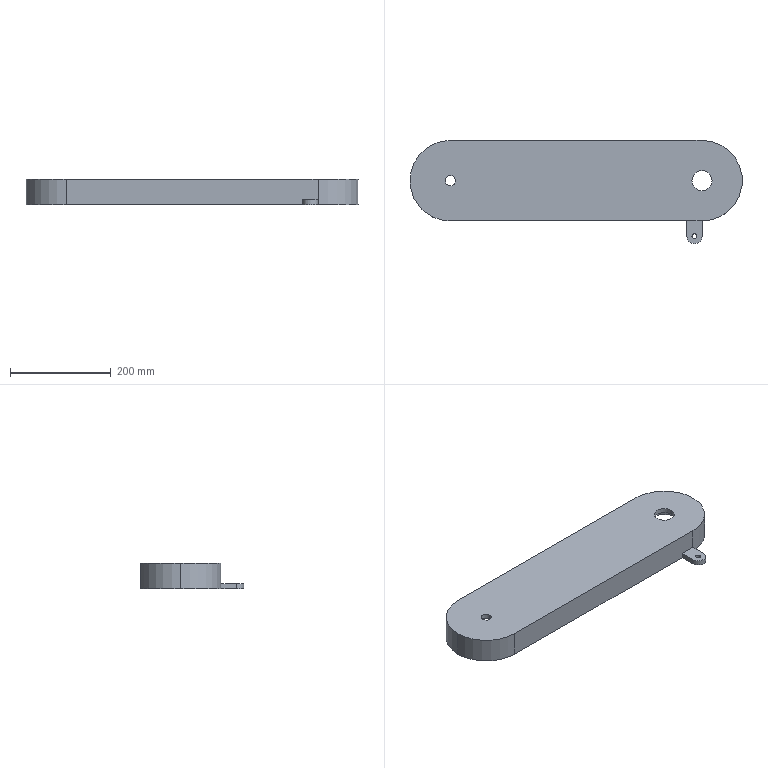Part | SolidWorks | features ICE 2, Extrusion 1 | 1 solid | 23 faces | box 660 x 205 x 50 mm | volume 1585598 mm3 | cylinder 13 | plane 10 | commonest cylinder face diameters 140 x3 160 x3 10 x2 20 x2 40 x2 30 x1
STEP:
#1=CARTESIAN_POINT('',(-10.,-110.,-30.));
#2=VERTEX_POINT('',#1);
#3=CARTESIAN_POINT('',(-20.,-110.,-30.));
#4=VERTEX_POINT('',#3);
#5=CARTESIAN_POINT('',(-15.,-110.,-30.));
#6=DIRECTION('',(0.,0.,-1.));
#7=DIRECTION('',(1.,0.,0.));
#8=AXIS2_PLACEMENT_3D('',#5,#6,#7);
#9=CIRCLE('',#8,5.);
#10=EDGE_CURVE('',#2,#4,#9,.T.);
#11=ORIENTED_EDGE('',*,*,#10,.F.);
#12=CARTESIAN_POINT('',(-10.,-110.,-40.));
#13=VERTEX_POINT('',#12);
#14=CARTESIAN_POINT('',(-10.,-110.,-30.));
#15=DIRECTION('',(0.,0.,-1.));
#16=VECTOR('',#15,1000.);
#17=LINE('',#14,#16);
#18=EDGE_CURVE('',#2,#13,#17,.T.);
#19=ORIENTED_EDGE('',*,*,#18,.T.);
#20=CARTESIAN_POINT('',(-20.,-110.,-40.));
#21=VERTEX_POINT('',#20);
#22=CARTESIAN_POINT('',(-15.,-110.,-40.));
#23=DIRECTION('',(0.,0.,-1.));
#24=DIRECTION('',(1.,0.,0.));
#25=AXIS2_PLACEMENT_3D('',#22,#23,#24);
#26=CIRCLE('',#25,5.);
#27=EDGE_CURVE('',#13,#21,#26,.T.);
#28=ORIENTED_EDGE('',*,*,#27,.T.);
#29=CARTESIAN_POINT('',(-20.,-110.,-30.));
#30=DIRECTION('',(0.,0.,-1.));
#31=VECTOR('',#30,1000.);
#32=LINE('',#29,#31);
#33=EDGE_CURVE('',#4,#21,#32,.T.);
#34=ORIENTED_EDGE('',*,*,#33,.F.);
#35=EDGE_LOOP('',(#11,#19,#28,#34));
#36=FACE_OUTER_BOUND('',#35,.T.);
#37=CARTESIAN_POINT('',(-15.,-110.,-30.));
#38=DIRECTION('',(0.,0.,-1.));
#39=DIRECTION('',(-1.,0.,0.));
#40=AXIS2_PLACEMENT_3D('',#37,#38,#39);
#41=CYLINDRICAL_SURFACE('',#40,5.);
#42=ADVANCED_FACE('',(#36),#41,.F.);
#43=CARTESIAN_POINT('',(0.,70.,-40.));
#44=VERTEX_POINT('',#43);
#45=CARTESIAN_POINT('',(70.,0.,-40.));
#46=VERTEX_POINT('',#45);
#47=CARTESIAN_POINT('',(0.,0.,-40.));
#48=DIRECTION('',(0.,0.,-1.));
#49=DIRECTION('',(-1.,0.,0.));
#50=AXIS2_PLACEMENT_3D('',#47,#48,#49);
#51=CIRCLE('',#50,70.);
#52=EDGE_CURVE('',#44,#46,#51,.T.);
#53=ORIENTED_EDGE('',*,*,#52,.T.);
#54=CARTESIAN_POINT('',(70.,0.,0.));
#55=VERTEX_POINT('',#54);
#56=CARTESIAN_POINT('',(70.,0.,-40.));
#57=DIRECTION('',(0.,0.,1.));
#58=VECTOR('',#57,1000.);
#59=LINE('',#56,#58);
#60=EDGE_CURVE('',#46,#55,#59,.T.);
#61=ORIENTED_EDGE('',*,*,#60,.T.);
#62=CARTESIAN_POINT('',(0.,70.,0.));
#63=VERTEX_POINT('',#62);
#64=CARTESIAN_POINT('',(0.,0.,0.));
#65=DIRECTION('',(0.,0.,-1.));
#66=DIRECTION('',(-1.,0.,0.));
#67=AXIS2_PLACEMENT_3D('',#64,#65,#66);
#68=CIRCLE('',#67,70.);
#69=EDGE_CURVE('',#63,#55,#68,.T.);
#70=ORIENTED_EDGE('',*,*,#69,.F.);
#71=CARTESIAN_POINT('',(0.,70.,-40.));
#72=DIRECTION('',(0.,0.,1.));
#73=VECTOR('',#72,1000.);
#74=LINE('',#71,#73);
#75=EDGE_CURVE('',#44,#63,#74,.T.);
#76=ORIENTED_EDGE('',*,*,#75,.F.);
#77=EDGE_LOOP('',(#53,#61,#70,#76));
#78=FACE_OUTER_BOUND('',#77,.T.);
#79=CARTESIAN_POINT('',(0.,0.,-40.));
#80=DIRECTION('',(0.,0.,1.));
#81=DIRECTION('',(1.,0.,0.));
#82=AXIS2_PLACEMENT_3D('',#79,#80,#81);
#83=CYLINDRICAL_SURFACE('',#82,70.);
#84=ADVANCED_FACE('',(#78),#83,.F.);
#85=CARTESIAN_POINT('',(-510.,0.,10.));
#86=VERTEX_POINT('',#85);
#87=CARTESIAN_POINT('',(-490.,0.,10.));
#88=VERTEX_POINT('',#87);
#89=CARTESIAN_POINT('',(-500.,0.,10.));
#90=DIRECTION('',(0.,0.,1.));
#91=DIRECTION('',(1.,0.,0.));
#92=AXIS2_PLACEMENT_3D('',#89,#90,#91);
#93=CIRCLE('',#92,10.);
#94=EDGE_CURVE('',#86,#88,#93,.T.);
#95=ORIENTED_EDGE('',*,*,#94,.T.);
#96=CARTESIAN_POINT('',(-490.,0.,0.));
#97=VERTEX_POINT('',#96);
#98=CARTESIAN_POINT('',(-490.,0.,10.));
#99=DIRECTION('',(0.,0.,-1.));
#100=VECTOR('',#99,1000.);
#101=LINE('',#98,#100);
#102=EDGE_CURVE('',#88,#97,#101,.T.);
#103=ORIENTED_EDGE('',*,*,#102,.T.);
#104=CARTESIAN_POINT('',(-510.,0.,0.));
#105=VERTEX_POINT('',#104);
#106=CARTESIAN_POINT('',(-500.,0.,0.));
#107=DIRECTION('',(0.,0.,1.));
#108=DIRECTION('',(1.,0.,0.));
#109=AXIS2_PLACEMENT_3D('',#106,#107,#108);
#110=CIRCLE('',#109,10.);
#111=EDGE_CURVE('',#105,#97,#110,.T.);
#112=ORIENTED_EDGE('',*,*,#111,.F.);
#113=CARTESIAN_POINT('',(-510.,0.,10.));
#114=DIRECTION('',(0.,0.,-1.));
#115=VECTOR('',#114,1000.);
#116=LINE('',#113,#115);
#117=EDGE_CURVE('',#86,#105,#116,.T.);
#118=ORIENTED_EDGE('',*,*,#117,.F.);
#119=EDGE_LOOP('',(#95,#103,#112,#118));
#120=FACE_OUTER_BOUND('',#119,.T.);
#121=CARTESIAN_POINT('',(-500.,0.,10.));
#122=DIRECTION('',(0.,0.,-1.));
#123=DIRECTION('',(-1.,0.,0.));
#124=AXIS2_PLACEMENT_3D('',#121,#122,#123);
#125=CYLINDRICAL_SURFACE('',#124,10.);
#126=ADVANCED_FACE('',(#120),#125,.F.);
#127=CARTESIAN_POINT('',(-20.,0.,10.));
#128=VERTEX_POINT('',#127);
#129=CARTESIAN_POINT('',(20.,0.,10.));
#130=VERTEX_POINT('',#129);
#131=CARTESIAN_POINT('',(0.,0.,10.));
#132=DIRECTION('',(0.,0.,1.));
#133=DIRECTION('',(1.,0.,0.));
#134=AXIS2_PLACEMENT_3D('',#131,#132,#133);
#135=CIRCLE('',#134,20.);
#136=EDGE_CURVE('',#128,#130,#135,.T.);
#137=ORIENTED_EDGE('',*,*,#136,.T.);
#138=CARTESIAN_POINT('',(20.,0.,0.));
#139=VERTEX_POINT('',#138);
#140=CARTESIAN_POINT('',(20.,0.,10.));
#141=DIRECTION('',(0.,0.,-1.));
#142=VECTOR('',#141,1000.);
#143=LINE('',#140,#142);
#144=EDGE_CURVE('',#130,#139,#143,.T.);
#145=ORIENTED_EDGE('',*,*,#144,.T.);
#146=CARTESIAN_POINT('',(-20.,0.,0.));
#147=VERTEX_POINT('',#146);
#148=CARTESIAN_POINT('',(0.,0.,0.));
#149=DIRECTION('',(0.,0.,1.));
#150=DIRECTION('',(1.,0.,0.));
#151=AXIS2_PLACEMENT_3D('',#148,#149,#150);
#152=CIRCLE('',#151,20.);
#153=EDGE_CURVE('',#147,#139,#152,.T.);
#154=ORIENTED_EDGE('',*,*,#153,.F.);
#155=CARTESIAN_POINT('',(-20.,0.,10.));
#156=DIRECTION('',(0.,0.,-1.));
#157=VECTOR('',#156,1000.);
#158=LINE('',#155,#157);
#159=EDGE_CURVE('',#128,#147,#158,.T.);
#160=ORIENTED_EDGE('',*,*,#159,.F.);
#161=EDGE_LOOP('',(#137,#145,#154,#160));
#162=FACE_OUTER_BOUND('',#161,.T.);
#163=CARTESIAN_POINT('',(0.,0.,10.));
#164=DIRECTION('',(0.,0.,-1.));
#165=DIRECTION('',(-1.,0.,0.));
#166=AXIS2_PLACEMENT_3D('',#163,#164,#165);
#167=CYLINDRICAL_SURFACE('',#166,20.);
#168=ADVANCED_FACE('',(#162),#167,.F.);
#169=CARTESIAN_POINT('',(-580.,0.,10.));
#170=VERTEX_POINT('',#169);
#171=CARTESIAN_POINT('',(-500.,-80.,10.));
#172=VERTEX_POINT('',#171);
#173=CARTESIAN_POINT('',(-500.,0.,10.));
#174=DIRECTION('',(0.,0.,1.));
#175=DIRECTION('',(1.,0.,0.));
#176=AXIS2_PLACEMENT_3D('',#173,#174,#175);
#177=CIRCLE('',#176,80.);
#178=EDGE_CURVE('',#170,#172,#177,.T.);
#179=ORIENTED_EDGE('',*,*,#178,.F.);
#180=CARTESIAN_POINT('',(-580.,0.,-40.));
#181=VERTEX_POINT('',#180);
#182=CARTESIAN_POINT('',(-580.,0.,10.));
#183=DIRECTION('',(0.,0.,-1.));
#184=VECTOR('',#183,1000.);
#185=LINE('',#182,#184);
#186=EDGE_CURVE('',#170,#181,#185,.T.);
#187=ORIENTED_EDGE('',*,*,#186,.T.);
#188=CARTESIAN_POINT('',(-500.,-80.,-40.));
#189=VERTEX_POINT('',#188);
#190=CARTESIAN_POINT('',(-500.,0.,-40.));
#191=DIRECTION('',(0.,0.,-1.));
#192=DIRECTION('',(-1.,0.,0.));
#193=AXIS2_PLACEMENT_3D('',#190,#191,#192);
#194=CIRCLE('',#193,80.);
#195=EDGE_CURVE('',#189,#181,#194,.T.);
#196=ORIENTED_EDGE('',*,*,#195,.F.);
#197=CARTESIAN_POINT('',(-500.,-80.,10.));
#198=DIRECTION('',(0.,0.,-1.));
#199=VECTOR('',#198,1000.);
#200=LINE('',#197,#199);
#201=EDGE_CURVE('',#172,#189,#200,.T.);
#202=ORIENTED_EDGE('',*,*,#201,.F.);
#203=EDGE_LOOP('',(#179,#187,#196,#202));
#204=FACE_OUTER_BOUND('',#203,.T.);
#205=CARTESIAN_POINT('',(-500.,0.,10.));
#206=DIRECTION('',(0.,0.,-1.));
#207=DIRECTION('',(-1.,0.,0.));
#208=AXIS2_PLACEMENT_3D('',#205,#206,#207);
#209=CYLINDRICAL_SURFACE('',#208,80.);
#210=ADVANCED_FACE('',(#204),#209,.T.);
#211=ORIENTED_EDGE('',*,*,#136,.F.);
#212=CARTESIAN_POINT('',(0.,0.,10.));
#213=DIRECTION('',(0.,0.,1.));
#214=DIRECTION('',(1.,0.,0.));
#215=AXIS2_PLACEMENT_3D('',#212,#213,#214);
#216=CIRCLE('',#215,20.);
#217=EDGE_CURVE('',#130,#128,#216,.T.);
#218=ORIENTED_EDGE('',*,*,#217,.F.);
#219=EDGE_LOOP('',(#211,#218));
#220=FACE_BOUND('',#219,.T.);
#221=CARTESIAN_POINT('',(0.,-80.,10.));
#222=VERTEX_POINT('',#221);
#223=CARTESIAN_POINT('',(0.,80.,10.));
#224=VERTEX_POINT('',#223);
#225=CARTESIAN_POINT('',(0.,0.,10.));
#226=DIRECTION('',(0.,0.,1.));
#227=DIRECTION('',(1.,0.,0.));
#228=AXIS2_PLACEMENT_3D('',#225,#226,#227);
#229=CIRCLE('',#228,80.);
#230=EDGE_CURVE('',#222,#224,#229,.T.);
#231=ORIENTED_EDGE('',*,*,#230,.T.);
#232=CARTESIAN_POINT('',(-500.,80.,10.));
#233=VERTEX_POINT('',#232);
#234=CARTESIAN_POINT('',(0.,80.,10.));
#235=DIRECTION('',(-1.,0.,0.));
#236=VECTOR('',#235,1000.);
#237=LINE('',#234,#236);
#238=EDGE_CURVE('',#224,#233,#237,.T.);
#239=ORIENTED_EDGE('',*,*,#238,.T.);
#240=CARTESIAN_POINT('',(-500.,0.,10.));
#241=DIRECTION('',(0.,0.,1.));
#242=DIRECTION('',(1.,0.,0.));
#243=AXIS2_PLACEMENT_3D('',#240,#241,#242);
#244=CIRCLE('',#243,80.);
#245=EDGE_CURVE('',#233,#170,#244,.T.);
#246=ORIENTED_EDGE('',*,*,#245,.T.);
#247=ORIENTED_EDGE('',*,*,#178,.T.);
#248=CARTESIAN_POINT('',(-500.,-80.,10.));
#249=DIRECTION('',(1.,0.,0.));
#250=VECTOR('',#249,1000.);
#251=LINE('',#248,#250);
#252=EDGE_CURVE('',#172,#222,#251,.T.);
#253=ORIENTED_EDGE('',*,*,#252,.T.);
#254=EDGE_LOOP('',(#231,#239,#246,#247,#253));
#255=FACE_OUTER_BOUND('',#254,.T.);
#256=ORIENTED_EDGE('',*,*,#94,.F.);
#257=CARTESIAN_POINT('',(-500.,0.,10.));
#258=DIRECTION('',(0.,0.,1.));
#259=DIRECTION('',(1.,0.,0.));
#260=AXIS2_PLACEMENT_3D('',#257,#258,#259);
#261=CIRCLE('',#260,10.);
#262=EDGE_CURVE('',#88,#86,#261,.T.);
#263=ORIENTED_EDGE('',*,*,#262,.F.);
#264=EDGE_LOOP('',(#256,#263));
#265=FACE_BOUND('',#264,.T.);
#266=CARTESIAN_POINT('',(0.,0.,10.));
#267=DIRECTION('',(0.,0.,1.));
#268=DIRECTION('',(1.,0.,0.));
#269=AXIS2_PLACEMENT_3D('',#266,#267,#268);
#270=PLANE('',#269);
#271=ADVANCED_FACE('',(#220,#255,#265),#270,.T.);
#272=CARTESIAN_POINT('',(-500.,70.,0.));
#273=VERTEX_POINT('',#272);
#274=CARTESIAN_POINT('',(-500.,70.,0.));
#275=DIRECTION('',(1.,0.,0.));
#276=VECTOR('',#275,1000.);
#277=LINE('',#274,#276);
#278=EDGE_CURVE('',#273,#63,#277,.T.);
#279=ORIENTED_EDGE('',*,*,#278,.T.);
#280=ORIENTED_EDGE('',*,*,#69,.T.);
#281=CARTESIAN_POINT('',(0.,-70.,0.));
#282=VERTEX_POINT('',#281);
#283=CARTESIAN_POINT('',(0.,0.,0.));
#284=DIRECTION('',(0.,0.,-1.));
#285=DIRECTION('',(-1.,0.,0.));
#286=AXIS2_PLACEMENT_3D('',#283,#284,#285);
#287=CIRCLE('',#286,70.);
#288=EDGE_CURVE('',#55,#282,#287,.T.);
#289=ORIENTED_EDGE('',*,*,#288,.T.);
#290=CARTESIAN_POINT('',(-500.,-70.,0.));
#291=VERTEX_POINT('',#290);
#292=CARTESIAN_POINT('',(0.,-70.,0.));
#293=DIRECTION('',(-1.,0.,0.));
#294=VECTOR('',#293,1000.);
#295=LINE('',#292,#294);
#296=EDGE_CURVE('',#282,#291,#295,.T.);
#297=ORIENTED_EDGE('',*,*,#296,.T.);
#298=CARTESIAN_POINT('',(-500.,0.,0.));
#299=DIRECTION('',(0.,0.,-1.));
#300=DIRECTION('',(-1.,0.,0.));
#301=AXIS2_PLACEMENT_3D('',#298,#299,#300);
#302=CIRCLE('',#301,70.);
#303=EDGE_CURVE('',#291,#273,#302,.T.);
#304=ORIENTED_EDGE('',*,*,#303,.T.);
#305=EDGE_LOOP('',(#279,#280,#289,#297,#304));
#306=FACE_OUTER_BOUND('',#305,.T.);
#307=ORIENTED_EDGE('',*,*,#153,.T.);
#308=CARTESIAN_POINT('',(0.,0.,0.));
#309=DIRECTION('',(0.,0.,1.));
#310=DIRECTION('',(1.,0.,0.));
#311=AXIS2_PLACEMENT_3D('',#308,#309,#310);
#312=CIRCLE('',#311,20.);
#313=EDGE_CURVE('',#139,#147,#312,.T.);
#314=ORIENTED_EDGE('',*,*,#313,.T.);
#315=EDGE_LOOP('',(#307,#314));
#316=FACE_BOUND('',#315,.T.);
#317=ORIENTED_EDGE('',*,*,#111,.T.);
#318=CARTESIAN_POINT('',(-500.,0.,0.));
#319=DIRECTION('',(0.,0.,1.));
#320=DIRECTION('',(1.,0.,0.));
#321=AXIS2_PLACEMENT_3D('',#318,#319,#320);
#322=CIRCLE('',#321,10.);
#323=EDGE_CURVE('',#97,#105,#322,.T.);
#324=ORIENTED_EDGE('',*,*,#323,.T.);
#325=EDGE_LOOP('',(#317,#324));
#326=FACE_BOUND('',#325,.T.);
#327=CARTESIAN_POINT('',(0.,0.,0.));
#328=DIRECTION('',(0.,0.,1.));
#329=DIRECTION('',(1.,0.,0.));
#330=AXIS2_PLACEMENT_3D('',#327,#328,#329);
#331=PLANE('',#330);
#332=ADVANCED_FACE('',(#306,#316,#326),#331,.F.);
#333=CARTESIAN_POINT('',(0.,-80.,-30.));
#334=VERTEX_POINT('',#333);
#335=CARTESIAN_POINT('',(0.,-80.,10.));
#336=DIRECTION('',(0.,0.,-1.));
#337=VECTOR('',#336,1000.);
#338=LINE('',#335,#337);
#339=EDGE_CURVE('',#222,#334,#338,.T.);
#340=ORIENTED_EDGE('',*,*,#339,.T.);
#341=CARTESIAN_POINT('',(0.,-80.,-40.));
#342=VERTEX_POINT('',#341);
#343=CARTESIAN_POINT('',(0.,-80.,-30.));
#344=DIRECTION('',(0.,0.,-1.));
#345=VECTOR('',#344,1000.);
#346=LINE('',#343,#345);
#347=EDGE_CURVE('',#334,#342,#346,.T.);
#348=ORIENTED_EDGE('',*,*,#347,.T.);
#349=CARTESIAN_POINT('',(0.,80.,-40.));
#350=VERTEX_POINT('',#349);
#351=CARTESIAN_POINT('',(0.,0.,-40.));
#352=DIRECTION('',(0.,0.,-1.));
#353=DIRECTION('',(-1.,0.,0.));
#354=AXIS2_PLACEMENT_3D('',#351,#352,#353);
#355=CIRCLE('',#354,80.);
#356=EDGE_CURVE('',#350,#342,#355,.T.);
#357=ORIENTED_EDGE('',*,*,#356,.F.);
#358=CARTESIAN_POINT('',(0.,80.,10.));
#359=DIRECTION('',(0.,0.,-1.));
#360=VECTOR('',#359,1000.);
#361=LINE('',#358,#360);
#362=EDGE_CURVE('',#224,#350,#361,.T.);
#363=ORIENTED_EDGE('',*,*,#362,.F.);
#364=ORIENTED_EDGE('',*,*,#230,.F.);
#365=EDGE_LOOP('',(#340,#348,#357,#363,#364));
#366=FACE_OUTER_BOUND('',#365,.T.);
#367=CARTESIAN_POINT('',(0.,0.,10.));
#368=DIRECTION('',(0.,0.,-1.));
#369=DIRECTION('',(-1.,0.,0.));
#370=AXIS2_PLACEMENT_3D('',#367,#368,#369);
#371=CYLINDRICAL_SURFACE('',#370,80.);
#372=ADVANCED_FACE('',(#366),#371,.T.);
#373=ORIENTED_EDGE('',*,*,#362,.T.);
#374=CARTESIAN_POINT('',(-500.,80.,-40.));
#375=VERTEX_POINT('',#374);
#376=CARTESIAN_POINT('',(-500.,80.,-40.));
#377=DIRECTION('',(1.,0.,0.));
#378=VECTOR('',#377,1000.);
#379=LINE('',#376,#378);
#380=EDGE_CURVE('',#375,#350,#379,.T.);
#381=ORIENTED_EDGE('',*,*,#380,.F.);
#382=CARTESIAN_POINT('',(-500.,80.,10.));
#383=DIRECTION('',(0.,0.,-1.));
#384=VECTOR('',#383,1000.);
#385=LINE('',#382,#384);
#386=EDGE_CURVE('',#233,#375,#385,.T.);
#387=ORIENTED_EDGE('',*,*,#386,.F.);
#388=ORIENTED_EDGE('',*,*,#238,.F.);
#389=EDGE_LOOP('',(#373,#381,#387,#388));
#390=FACE_OUTER_BOUND('',#389,.T.);
#391=CARTESIAN_POINT('',(0.,80.,10.));
#392=DIRECTION('',(0.,-1.,0.));
#393=DIRECTION('',(1.,0.,0.));
#394=AXIS2_PLACEMENT_3D('',#391,#392,#393);
#395=PLANE('',#394);
#396=ADVANCED_FACE('',(#390),#395,.F.);
#397=ORIENTED_EDGE('',*,*,#186,.F.);
#398=ORIENTED_EDGE('',*,*,#245,.F.);
#399=ORIENTED_EDGE('',*,*,#386,.T.);
#400=CARTESIAN_POINT('',(-500.,0.,-40.));
#401=DIRECTION('',(0.,0.,-1.));
#402=DIRECTION('',(-1.,0.,0.));
#403=AXIS2_PLACEMENT_3D('',#400,#401,#402);
#404=CIRCLE('',#403,80.);
#405=EDGE_CURVE('',#181,#375,#404,.T.);
#406=ORIENTED_EDGE('',*,*,#405,.F.);
#407=EDGE_LOOP('',(#397,#398,#399,#406));
#408=FACE_OUTER_BOUND('',#407,.T.);
#409=CARTESIAN_POINT('',(-500.,0.,10.));
#410=DIRECTION('',(0.,0.,-1.));
#411=DIRECTION('',(-1.,0.,0.));
#412=AXIS2_PLACEMENT_3D('',#409,#410,#411);
#413=CYLINDRICAL_SURFACE('',#412,80.);
#414=ADVANCED_FACE('',(#408),#413,.T.);
#415=CARTESIAN_POINT('',(-30.,-80.,-40.));
#416=VERTEX_POINT('',#415);
#417=CARTESIAN_POINT('',(0.,-80.,-40.));
#418=DIRECTION('',(-1.,0.,0.));
#419=VECTOR('',#418,1000.);
#420=LINE('',#417,#419);
#421=EDGE_CURVE('',#416,#189,#420,.T.);
#422=ORIENTED_EDGE('',*,*,#421,.F.);
#423=CARTESIAN_POINT('',(-30.,-80.,-30.));
#424=VERTEX_POINT('',#423);
#425=CARTESIAN_POINT('',(-30.,-80.,-30.));
#426=DIRECTION('',(0.,0.,-1.));
#427=VECTOR('',#426,1000.);
#428=LINE('',#425,#427);
#429=EDGE_CURVE('',#424,#416,#428,.T.);
#430=ORIENTED_EDGE('',*,*,#429,.F.);
#431=CARTESIAN_POINT('',(0.,-80.,-30.));
#432=DIRECTION('',(1.,0.,0.));
#433=VECTOR('',#432,1000.);
#434=LINE('',#431,#433);
#435=EDGE_CURVE('',#424,#334,#434,.T.);
#436=ORIENTED_EDGE('',*,*,#435,.T.);
#437=ORIENTED_EDGE('',*,*,#339,.F.);
#438=ORIENTED_EDGE('',*,*,#252,.F.);
#439=ORIENTED_EDGE('',*,*,#201,.T.);
#440=EDGE_LOOP('',(#422,#430,#436,#437,#438,#439));
#441=FACE_OUTER_BOUND('',#440,.T.);
#442=CARTESIAN_POINT('',(-500.,-80.,10.));
#443=DIRECTION('',(0.,1.,0.));
#444=DIRECTION('',(0.,0.,1.));
#445=AXIS2_PLACEMENT_3D('',#442,#443,#444);
#446=PLANE('',#445);
#447=ADVANCED_FACE('',(#441),#446,.F.);
#448=ORIENTED_EDGE('',*,*,#144,.F.);
#449=ORIENTED_EDGE('',*,*,#217,.T.);
#450=ORIENTED_EDGE('',*,*,#159,.T.);
#451=ORIENTED_EDGE('',*,*,#313,.F.);
#452=EDGE_LOOP('',(#448,#449,#450,#451));
#453=FACE_OUTER_BOUND('',#452,.T.);
#454=CARTESIAN_POINT('',(0.,0.,10.));
#455=DIRECTION('',(0.,0.,-1.));
#456=DIRECTION('',(-1.,0.,0.));
#457=AXIS2_PLACEMENT_3D('',#454,#455,#456);
#458=CYLINDRICAL_SURFACE('',#457,20.);
#459=ADVANCED_FACE('',(#453),#458,.F.);
#460=ORIENTED_EDGE('',*,*,#102,.F.);
#461=ORIENTED_EDGE('',*,*,#262,.T.);
#462=ORIENTED_EDGE('',*,*,#117,.T.);
#463=ORIENTED_EDGE('',*,*,#323,.F.);
#464=EDGE_LOOP('',(#460,#461,#462,#463));
#465=FACE_OUTER_BOUND('',#464,.T.);
#466=CARTESIAN_POINT('',(-500.,0.,10.));
#467=DIRECTION('',(0.,0.,-1.));
#468=DIRECTION('',(-1.,0.,0.));
#469=AXIS2_PLACEMENT_3D('',#466,#467,#468);
#470=CYLINDRICAL_SURFACE('',#469,10.);
#471=ADVANCED_FACE('',(#465),#470,.F.);
#472=ORIENTED_EDGE('',*,*,#356,.T.);
#473=CARTESIAN_POINT('',(0.,-110.,-40.));
#474=VERTEX_POINT('',#473);
#475=CARTESIAN_POINT('',(0.,-110.,-40.));
#476=DIRECTION('',(0.,-1.,0.));
#477=VECTOR('',#476,1000.);
#478=LINE('',#475,#477);
#479=EDGE_CURVE('',#342,#474,#478,.T.);
#480=ORIENTED_EDGE('',*,*,#479,.T.);
#481=CARTESIAN_POINT('',(-30.,-110.,-40.));
#482=VERTEX_POINT('',#481);
#483=CARTESIAN_POINT('',(-15.,-110.,-40.));
#484=DIRECTION('',(0.,0.,-1.));
#485=DIRECTION('',(1.,0.,0.));
#486=AXIS2_PLACEMENT_3D('',#483,#484,#485);
#487=CIRCLE('',#486,15.);
#488=EDGE_CURVE('',#474,#482,#487,.T.);
#489=ORIENTED_EDGE('',*,*,#488,.T.);
#490=CARTESIAN_POINT('',(-30.,-110.,-40.));
#491=DIRECTION('',(0.,1.,0.));
#492=VECTOR('',#491,1000.);
#493=LINE('',#490,#492);
#494=EDGE_CURVE('',#482,#416,#493,.T.);
#495=ORIENTED_EDGE('',*,*,#494,.T.);
#496=ORIENTED_EDGE('',*,*,#421,.T.);
#497=ORIENTED_EDGE('',*,*,#195,.T.);
#498=ORIENTED_EDGE('',*,*,#405,.T.);
#499=ORIENTED_EDGE('',*,*,#380,.T.);
#500=EDGE_LOOP('',(#472,#480,#489,#495,#496,#497,#498,#499));
#501=FACE_OUTER_BOUND('',#500,.T.);
#502=CARTESIAN_POINT('',(0.,-70.,-40.));
#503=VERTEX_POINT('',#502);
#504=CARTESIAN_POINT('',(-500.,-70.,-40.));
#505=VERTEX_POINT('',#504);
#506=CARTESIAN_POINT('',(0.,-70.,-40.));
#507=DIRECTION('',(-1.,0.,0.));
#508=VECTOR('',#507,1000.);
#509=LINE('',#506,#508);
#510=EDGE_CURVE('',#503,#505,#509,.T.);
#511=ORIENTED_EDGE('',*,*,#510,.F.);
#512=CARTESIAN_POINT('',(0.,0.,-40.));
#513=DIRECTION('',(0.,0.,-1.));
#514=DIRECTION('',(-1.,0.,0.));
#515=AXIS2_PLACEMENT_3D('',#512,#513,#514);
#516=CIRCLE('',#515,70.);
#517=EDGE_CURVE('',#46,#503,#516,.T.);
#518=ORIENTED_EDGE('',*,*,#517,.F.);
#519=ORIENTED_EDGE('',*,*,#52,.F.);
#520=CARTESIAN_POINT('',(-500.,70.,-40.));
#521=VERTEX_POINT('',#520);
#522=CARTESIAN_POINT('',(-500.,70.,-40.));
#523=DIRECTION('',(1.,0.,0.));
#524=VECTOR('',#523,1000.);
#525=LINE('',#522,#524);
#526=EDGE_CURVE('',#521,#44,#525,.T.);
#527=ORIENTED_EDGE('',*,*,#526,.F.);
#528=CARTESIAN_POINT('',(-500.,0.,-40.));
#529=DIRECTION('',(0.,0.,-1.));
#530=DIRECTION('',(-1.,0.,0.));
#531=AXIS2_PLACEMENT_3D('',#528,#529,#530);
#532=CIRCLE('',#531,70.);
#533=EDGE_CURVE('',#505,#521,#532,.T.);
#534=ORIENTED_EDGE('',*,*,#533,.F.);
#535=EDGE_LOOP('',(#511,#518,#519,#527,#534));
#536=FACE_BOUND('',#535,.T.);
#537=CARTESIAN_POINT('',(-15.,-110.,-40.));
#538=DIRECTION('',(0.,0.,-1.));
#539=DIRECTION('',(1.,0.,0.));
#540=AXIS2_PLACEMENT_3D('',#537,#538,#539);
#541=CIRCLE('',#540,5.);
#542=EDGE_CURVE('',#21,#13,#541,.T.);
#543=ORIENTED_EDGE('',*,*,#542,.F.);
#544=ORIENTED_EDGE('',*,*,#27,.F.);
#545=EDGE_LOOP('',(#543,#544));
#546=FACE_BOUND('',#545,.T.);
#547=CARTESIAN_POINT('',(0.,0.,-40.));
#548=DIRECTION('',(0.,0.,-1.));
#549=DIRECTION('',(-1.,0.,0.));
#550=AXIS2_PLACEMENT_3D('',#547,#548,#549);
#551=PLANE('',#550);
#552=ADVANCED_FACE('',(#501,#536,#546),#551,.T.);
#553=ORIENTED_EDGE('',*,*,#60,.F.);
#554=ORIENTED_EDGE('',*,*,#517,.T.);
#555=CARTESIAN_POINT('',(0.,-70.,-40.));
#556=DIRECTION('',(0.,0.,1.));
#557=VECTOR('',#556,1000.);
#558=LINE('',#555,#557);
#559=EDGE_CURVE('',#503,#282,#558,.T.);
#560=ORIENTED_EDGE('',*,*,#559,.T.);
#561=ORIENTED_EDGE('',*,*,#288,.F.);
#562=EDGE_LOOP('',(#553,#554,#560,#561));
#563=FACE_OUTER_BOUND('',#562,.T.);
#564=CARTESIAN_POINT('',(0.,0.,-40.));
#565=DIRECTION('',(0.,0.,1.));
#566=DIRECTION('',(1.,0.,0.));
#567=AXIS2_PLACEMENT_3D('',#564,#565,#566);
#568=CYLINDRICAL_SURFACE('',#567,70.);
#569=ADVANCED_FACE('',(#563),#568,.F.);
#570=ORIENTED_EDGE('',*,*,#296,.F.);
#571=ORIENTED_EDGE('',*,*,#559,.F.);
#572=ORIENTED_EDGE('',*,*,#510,.T.);
#573=CARTESIAN_POINT('',(-500.,-70.,-40.));
#574=DIRECTION('',(0.,0.,1.));
#575=VECTOR('',#574,1000.);
#576=LINE('',#573,#575);
#577=EDGE_CURVE('',#505,#291,#576,.T.);
#578=ORIENTED_EDGE('',*,*,#577,.T.);
#579=EDGE_LOOP('',(#570,#571,#572,#578));
#580=FACE_OUTER_BOUND('',#579,.T.);
#581=CARTESIAN_POINT('',(0.,-70.,-40.));
#582=DIRECTION('',(0.,1.,0.));
#583=DIRECTION('',(-1.,0.,0.));
#584=AXIS2_PLACEMENT_3D('',#581,#582,#583);
#585=PLANE('',#584);
#586=ADVANCED_FACE('',(#580),#585,.T.);
#587=ORIENTED_EDGE('',*,*,#303,.F.);
#588=ORIENTED_EDGE('',*,*,#577,.F.);
#589=ORIENTED_EDGE('',*,*,#533,.T.);
#590=CARTESIAN_POINT('',(-500.,70.,-40.));
#591=DIRECTION('',(0.,0.,1.));
#592=VECTOR('',#591,1000.);
#593=LINE('',#590,#592);
#594=EDGE_CURVE('',#521,#273,#593,.T.);
#595=ORIENTED_EDGE('',*,*,#594,.T.);
#596=EDGE_LOOP('',(#587,#588,#589,#595));
#597=FACE_OUTER_BOUND('',#596,.T.);
#598=CARTESIAN_POINT('',(-500.,0.,-40.));
#599=DIRECTION('',(0.,0.,1.));
#600=DIRECTION('',(1.,0.,0.));
#601=AXIS2_PLACEMENT_3D('',#598,#599,#600);
#602=CYLINDRICAL_SURFACE('',#601,70.);
#603=ADVANCED_FACE('',(#597),#602,.F.);
#604=ORIENTED_EDGE('',*,*,#278,.F.);
#605=ORIENTED_EDGE('',*,*,#594,.F.);
#606=ORIENTED_EDGE('',*,*,#526,.T.);
#607=ORIENTED_EDGE('',*,*,#75,.T.);
#608=EDGE_LOOP('',(#604,#605,#606,#607));
#609=FACE_OUTER_BOUND('',#608,.T.);
#610=CARTESIAN_POINT('',(-500.,70.,-40.));
#611=DIRECTION('',(0.,-1.,0.));
#612=DIRECTION('',(1.,0.,0.));
#613=AXIS2_PLACEMENT_3D('',#610,#611,#612);
#614=PLANE('',#613);
#615=ADVANCED_FACE('',(#609),#614,.T.);
#616=ORIENTED_EDGE('',*,*,#488,.F.);
#617=CARTESIAN_POINT('',(0.,-110.,-30.));
#618=VERTEX_POINT('',#617);
#619=CARTESIAN_POINT('',(0.,-110.,-30.));
#620=DIRECTION('',(0.,0.,-1.));
#621=VECTOR('',#620,1000.);
#622=LINE('',#619,#621);
#623=EDGE_CURVE('',#618,#474,#622,.T.);
#624=ORIENTED_EDGE('',*,*,#623,.F.);
#625=CARTESIAN_POINT('',(-30.,-110.,-30.));
#626=VERTEX_POINT('',#625);
#627=CARTESIAN_POINT('',(-15.,-110.,-30.));
#628=DIRECTION('',(0.,0.,-1.));
#629=DIRECTION('',(1.,0.,0.));
#630=AXIS2_PLACEMENT_3D('',#627,#628,#629);
#631=CIRCLE('',#630,15.);
#632=EDGE_CURVE('',#618,#626,#631,.T.);
#633=ORIENTED_EDGE('',*,*,#632,.T.);
#634=CARTESIAN_POINT('',(-30.,-110.,-30.));
#635=DIRECTION('',(0.,0.,-1.));
#636=VECTOR('',#635,1000.);
#637=LINE('',#634,#636);
#638=EDGE_CURVE('',#626,#482,#637,.T.);
#639=ORIENTED_EDGE('',*,*,#638,.T.);
#640=EDGE_LOOP('',(#616,#624,#633,#639));
#641=FACE_OUTER_BOUND('',#640,.T.);
#642=CARTESIAN_POINT('',(-15.,-110.,-30.));
#643=DIRECTION('',(0.,0.,-1.));
#644=DIRECTION('',(-1.,0.,0.));
#645=AXIS2_PLACEMENT_3D('',#642,#643,#644);
#646=CYLINDRICAL_SURFACE('',#645,15.);
#647=ADVANCED_FACE('',(#641),#646,.T.);
#648=ORIENTED_EDGE('',*,*,#479,.F.);
#649=ORIENTED_EDGE('',*,*,#347,.F.);
#650=CARTESIAN_POINT('',(0.,-110.,-30.));
#651=DIRECTION('',(0.,-1.,0.));
#652=VECTOR('',#651,1000.);
#653=LINE('',#650,#652);
#654=EDGE_CURVE('',#334,#618,#653,.T.);
#655=ORIENTED_EDGE('',*,*,#654,.T.);
#656=ORIENTED_EDGE('',*,*,#623,.T.);
#657=EDGE_LOOP('',(#648,#649,#655,#656));
#658=FACE_OUTER_BOUND('',#657,.T.);
#659=CARTESIAN_POINT('',(0.,-110.,-30.));
#660=DIRECTION('',(1.,0.,0.));
#661=DIRECTION('',(0.,1.,0.));
#662=AXIS2_PLACEMENT_3D('',#659,#660,#661);
#663=PLANE('',#662);
#664=ADVANCED_FACE('',(#658),#663,.T.);
#665=ORIENTED_EDGE('',*,*,#494,.F.);
#666=ORIENTED_EDGE('',*,*,#638,.F.);
#667=CARTESIAN_POINT('',(-30.,-110.,-30.));
#668=DIRECTION('',(0.,1.,0.));
#669=VECTOR('',#668,1000.);
#670=LINE('',#667,#669);
#671=EDGE_CURVE('',#626,#424,#670,.T.);
#672=ORIENTED_EDGE('',*,*,#671,.T.);
#673=ORIENTED_EDGE('',*,*,#429,.T.);
#674=EDGE_LOOP('',(#665,#666,#672,#673));
#675=FACE_OUTER_BOUND('',#674,.T.);
#676=CARTESIAN_POINT('',(-30.,-110.,-30.));
#677=DIRECTION('',(-1.,0.,0.));
#678=DIRECTION('',(0.,-1.,0.));
#679=AXIS2_PLACEMENT_3D('',#676,#677,#678);
#680=PLANE('',#679);
#681=ADVANCED_FACE('',(#675),#680,.T.);
#682=CARTESIAN_POINT('',(-15.,-110.,-30.));
#683=DIRECTION('',(0.,0.,-1.));
#684=DIRECTION('',(1.,0.,0.));
#685=AXIS2_PLACEMENT_3D('',#682,#683,#684);
#686=CIRCLE('',#685,5.);
#687=EDGE_CURVE('',#4,#2,#686,.T.);
#688=ORIENTED_EDGE('',*,*,#687,.T.);
#689=ORIENTED_EDGE('',*,*,#10,.T.);
#690=EDGE_LOOP('',(#688,#689));
#691=FACE_BOUND('',#690,.T.);
#692=ORIENTED_EDGE('',*,*,#632,.F.);
#693=ORIENTED_EDGE('',*,*,#654,.F.);
#694=ORIENTED_EDGE('',*,*,#435,.F.);
#695=ORIENTED_EDGE('',*,*,#671,.F.);
#696=EDGE_LOOP('',(#692,#693,#694,#695));
#697=FACE_OUTER_BOUND('',#696,.T.);
#698=CARTESIAN_POINT('',(-15.,-110.,-30.));
#699=DIRECTION('',(0.,0.,1.));
#700=DIRECTION('',(1.,0.,0.));
#701=AXIS2_PLACEMENT_3D('',#698,#699,#700);
#702=PLANE('',#701);
#703=ADVANCED_FACE('',(#691,#697),#702,.T.);
#704=ORIENTED_EDGE('',*,*,#18,.F.);
#705=ORIENTED_EDGE('',*,*,#687,.F.);
#706=ORIENTED_EDGE('',*,*,#33,.T.);
#707=ORIENTED_EDGE('',*,*,#542,.T.);
#708=EDGE_LOOP('',(#704,#705,#706,#707));
#709=FACE_OUTER_BOUND('',#708,.T.);
#710=CARTESIAN_POINT('',(-15.,-110.,-30.));
#711=DIRECTION('',(0.,0.,-1.));
#712=DIRECTION('',(-1.,0.,0.));
#713=AXIS2_PLACEMENT_3D('',#710,#711,#712);
#714=CYLINDRICAL_SURFACE('',#713,5.);
#715=ADVANCED_FACE('',(#709),#714,.F.);
#716=CLOSED_SHELL('',(#42,#84,#126,#168,#210,#271,#332,#372,#396,#414,#447,#459,#471,#552,#569,#586,#603,#615,#647,#664,#681,#703,#715));
#717=MANIFOLD_SOLID_BREP('',#716);
#718=CARTESIAN_POINT('',(0.,0.,0.));
#719=DIRECTION('',(0.,0.,1.));
#720=DIRECTION('',(1.,0.,0.));
#721=AXIS2_PLACEMENT_3D('',#718,#719,#720);
#722=(LENGTH_UNIT()NAMED_UNIT(*)SI_UNIT(.MILLI.,.METRE.));
#723=UNCERTAINTY_MEASURE_WITH_UNIT(LENGTH_MEASURE(0.00001),#722,'','');
#724=(NAMED_UNIT(*)PLANE_ANGLE_UNIT()SI_UNIT($,.RADIAN.));
#725=(NAMED_UNIT(*)SI_UNIT($,.STERADIAN.)SOLID_ANGLE_UNIT());
#726=(GEOMETRIC_REPRESENTATION_CONTEXT(3)GLOBAL_UNCERTAINTY_ASSIGNED_CONTEXT((#723))GLOBAL_UNIT_ASSIGNED_CONTEXT((#722,#724,#725))REPRESENTATION_CONTEXT('',''));
#727=ADVANCED_BREP_SHAPE_REPRESENTATION('',(#717,#721),#726);